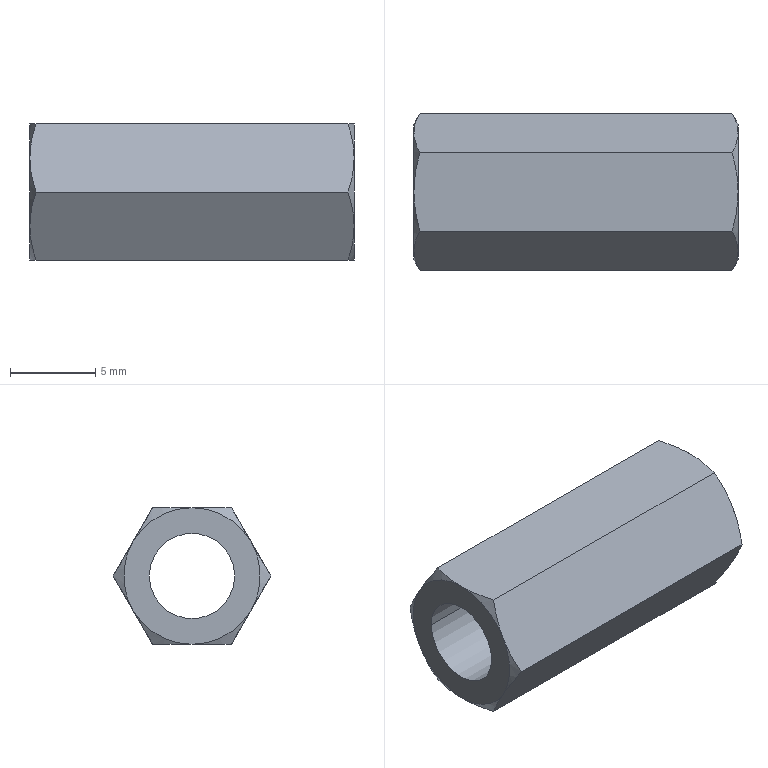Part | STEP file | PLSFB8-19.0-2 | 1 solid | 22 faces | box 19 x 9.238 x 8 mm | volume 678.916 mm3 | cone 12 | plane 8 | cylinder 2 | commonest cylinder face diameters 5 x2
STEP:
#1=CARTESIAN_POINT('',(0.,2.5,0.));
#2=VERTEX_POINT('',#1);
#3=CARTESIAN_POINT('',(0.,-2.5,0.));
#4=VERTEX_POINT('',#3);
#5=CARTESIAN_POINT('',(0.,0.,0.));
#6=DIRECTION('',(1.,0.,0.));
#7=DIRECTION('',(0.,1.,0.));
#8=AXIS2_PLACEMENT_3D('',#5,#6,#7);
#9=CIRCLE('',#8,2.5);
#10=EDGE_CURVE('',#2,#4,#9,.T.);
#11=ORIENTED_EDGE('',*,*,#10,.F.);
#12=CARTESIAN_POINT('',(19.,2.5,0.));
#13=VERTEX_POINT('',#12);
#14=CARTESIAN_POINT('',(19.,2.5,0.));
#15=DIRECTION('',(1.,0.,0.));
#16=VECTOR('',#15,1000.);
#17=LINE('',#14,#16);
#18=EDGE_CURVE('',#2,#13,#17,.T.);
#19=ORIENTED_EDGE('',*,*,#18,.T.);
#20=CARTESIAN_POINT('',(19.,-2.5,0.));
#21=VERTEX_POINT('',#20);
#22=CARTESIAN_POINT('',(19.,0.,0.));
#23=DIRECTION('',(-1.,0.,0.));
#24=DIRECTION('',(0.,-1.,0.));
#25=AXIS2_PLACEMENT_3D('',#22,#23,#24);
#26=CIRCLE('',#25,2.5);
#27=EDGE_CURVE('',#21,#13,#26,.T.);
#28=ORIENTED_EDGE('',*,*,#27,.F.);
#29=CARTESIAN_POINT('',(19.,-2.5,0.));
#30=DIRECTION('',(1.,0.,0.));
#31=VECTOR('',#30,1000.);
#32=LINE('',#29,#31);
#33=EDGE_CURVE('',#4,#21,#32,.T.);
#34=ORIENTED_EDGE('',*,*,#33,.F.);
#35=EDGE_LOOP('',(#11,#19,#28,#34));
#36=FACE_OUTER_BOUND('',#35,.T.);
#37=CARTESIAN_POINT('',(19.,0.,0.));
#38=DIRECTION('',(1.,0.,0.));
#39=DIRECTION('',(0.,-1.,0.));
#40=AXIS2_PLACEMENT_3D('',#37,#38,#39);
#41=CYLINDRICAL_SURFACE('',#40,2.5);
#42=ADVANCED_FACE('',(#36),#41,.F.);
#43=CARTESIAN_POINT('',(18.643,2.309,4.));
#44=VERTEX_POINT('',#43);
#45=CARTESIAN_POINT('',(19.,3.464,2.));
#46=VERTEX_POINT('',#45);
#47=CARTESIAN_POINT('',(18.643,2.309,4.));
#48=CARTESIAN_POINT('',(18.861,2.687,3.346));
#49=CARTESIAN_POINT('',(19.,3.071,2.681));
#50=CARTESIAN_POINT('',(19.,3.464,2.));
#51=B_SPLINE_CURVE_WITH_KNOTS('',3,(#47,#48,#49,#50),.UNSPECIFIED.,.F.,.F.,(4,4),(0.000000238,0.002337),.UNSPECIFIED.);
#52=EDGE_CURVE('',#44,#46,#51,.T.);
#53=ORIENTED_EDGE('',*,*,#52,.T.);
#54=CARTESIAN_POINT('',(18.643,4.619,0.));
#55=VERTEX_POINT('',#54);
#56=CARTESIAN_POINT('',(19.,3.464,2.));
#57=CARTESIAN_POINT('',(19.,3.66,1.661));
#58=CARTESIAN_POINT('',(18.966,3.856,1.322));
#59=CARTESIAN_POINT('',(18.841,4.24,0.6554));
#60=CARTESIAN_POINT('',(18.752,4.43,0.3264));
#61=CARTESIAN_POINT('',(18.643,4.619,0.));
#62=B_SPLINE_CURVE_WITH_KNOTS('',3,(#56,#57,#58,#59,#60,#61),.UNSPECIFIED.,.F.,.F.,(4,2,4),(0.002337,0.003501,0.004665),.UNSPECIFIED.);
#63=EDGE_CURVE('',#46,#55,#62,.T.);
#64=ORIENTED_EDGE('',*,*,#63,.T.);
#65=CARTESIAN_POINT('',(0.3573,4.619,0.));
#66=VERTEX_POINT('',#65);
#67=CARTESIAN_POINT('',(19.,4.619,0.));
#68=DIRECTION('',(-1.,0.,0.));
#69=VECTOR('',#68,1000.);
#70=LINE('',#67,#69);
#71=EDGE_CURVE('',#55,#66,#70,.T.);
#72=ORIENTED_EDGE('',*,*,#71,.T.);
#73=CARTESIAN_POINT('',(0.,3.464,2.));
#74=VERTEX_POINT('',#73);
#75=CARTESIAN_POINT('',(0.3573,4.619,0.));
#76=CARTESIAN_POINT('',(0.1392,4.241,0.6543));
#77=CARTESIAN_POINT('',(0.,3.858,1.319));
#78=CARTESIAN_POINT('',(0.,3.464,2.));
#79=B_SPLINE_CURVE_WITH_KNOTS('',3,(#75,#76,#77,#78),.UNSPECIFIED.,.F.,.F.,(4,4),(0.000000238,0.002337),.UNSPECIFIED.);
#80=EDGE_CURVE('',#66,#74,#79,.T.);
#81=ORIENTED_EDGE('',*,*,#80,.T.);
#82=CARTESIAN_POINT('',(0.3573,2.309,4.));
#83=VERTEX_POINT('',#82);
#84=CARTESIAN_POINT('',(0.,3.464,2.));
#85=CARTESIAN_POINT('',(0.,3.268,2.339));
#86=CARTESIAN_POINT('',(0.03421,3.072,2.678));
#87=CARTESIAN_POINT('',(0.1587,2.688,3.345));
#88=CARTESIAN_POINT('',(0.2485,2.498,3.674));
#89=CARTESIAN_POINT('',(0.3573,2.309,4.));
#90=B_SPLINE_CURVE_WITH_KNOTS('',3,(#84,#85,#86,#87,#88,#89),.UNSPECIFIED.,.F.,.F.,(4,2,4),(0.002337,0.003501,0.004665),.UNSPECIFIED.);
#91=EDGE_CURVE('',#74,#83,#90,.T.);
#92=ORIENTED_EDGE('',*,*,#91,.T.);
#93=CARTESIAN_POINT('',(19.,2.309,4.));
#94=DIRECTION('',(-1.,0.,0.));
#95=VECTOR('',#94,1000.);
#96=LINE('',#93,#95);
#97=EDGE_CURVE('',#44,#83,#96,.T.);
#98=ORIENTED_EDGE('',*,*,#97,.F.);
#99=EDGE_LOOP('',(#53,#64,#72,#81,#92,#98));
#100=FACE_OUTER_BOUND('',#99,.T.);
#101=CARTESIAN_POINT('',(19.,2.309,4.));
#102=DIRECTION('',(0.,-0.866,-0.5));
#103=DIRECTION('',(0.,-0.5,0.866));
#104=AXIS2_PLACEMENT_3D('',#101,#102,#103);
#105=PLANE('',#104);
#106=ADVANCED_FACE('',(#100),#105,.F.);
#107=CARTESIAN_POINT('',(19.,3.464,-2.));
#108=VERTEX_POINT('',#107);
#109=CARTESIAN_POINT('',(18.643,4.619,0.));
#110=CARTESIAN_POINT('',(18.861,4.241,-0.6543));
#111=CARTESIAN_POINT('',(19.,3.858,-1.319));
#112=CARTESIAN_POINT('',(19.,3.464,-2.));
#113=B_SPLINE_CURVE_WITH_KNOTS('',3,(#109,#110,#111,#112),.UNSPECIFIED.,.F.,.F.,(4,4),(0.000000238,0.002337),.UNSPECIFIED.);
#114=EDGE_CURVE('',#55,#108,#113,.T.);
#115=ORIENTED_EDGE('',*,*,#114,.T.);
#116=CARTESIAN_POINT('',(18.643,2.309,-4.));
#117=VERTEX_POINT('',#116);
#118=CARTESIAN_POINT('',(19.,3.464,-2.));
#119=CARTESIAN_POINT('',(19.,3.268,-2.339));
#120=CARTESIAN_POINT('',(18.966,3.072,-2.678));
#121=CARTESIAN_POINT('',(18.841,2.688,-3.345));
#122=CARTESIAN_POINT('',(18.752,2.498,-3.674));
#123=CARTESIAN_POINT('',(18.643,2.309,-4.));
#124=B_SPLINE_CURVE_WITH_KNOTS('',3,(#118,#119,#120,#121,#122,#123),.UNSPECIFIED.,.F.,.F.,(4,2,4),(0.002337,0.003501,0.004665),.UNSPECIFIED.);
#125=EDGE_CURVE('',#108,#117,#124,.T.);
#126=ORIENTED_EDGE('',*,*,#125,.T.);
#127=CARTESIAN_POINT('',(0.3573,2.309,-4.));
#128=VERTEX_POINT('',#127);
#129=CARTESIAN_POINT('',(19.,2.309,-4.));
#130=DIRECTION('',(-1.,0.,0.));
#131=VECTOR('',#130,1000.);
#132=LINE('',#129,#131);
#133=EDGE_CURVE('',#117,#128,#132,.T.);
#134=ORIENTED_EDGE('',*,*,#133,.T.);
#135=CARTESIAN_POINT('',(0.,3.464,-2.));
#136=VERTEX_POINT('',#135);
#137=CARTESIAN_POINT('',(0.3573,2.309,-4.));
#138=CARTESIAN_POINT('',(0.1392,2.687,-3.346));
#139=CARTESIAN_POINT('',(0.,3.071,-2.681));
#140=CARTESIAN_POINT('',(0.,3.464,-2.));
#141=B_SPLINE_CURVE_WITH_KNOTS('',3,(#137,#138,#139,#140),.UNSPECIFIED.,.F.,.F.,(4,4),(0.000000238,0.002337),.UNSPECIFIED.);
#142=EDGE_CURVE('',#128,#136,#141,.T.);
#143=ORIENTED_EDGE('',*,*,#142,.T.);
#144=CARTESIAN_POINT('',(0.,3.464,-2.));
#145=CARTESIAN_POINT('',(0.,3.66,-1.661));
#146=CARTESIAN_POINT('',(0.03421,3.856,-1.322));
#147=CARTESIAN_POINT('',(0.1587,4.24,-0.6554));
#148=CARTESIAN_POINT('',(0.2485,4.43,-0.3264));
#149=CARTESIAN_POINT('',(0.3573,4.619,0.));
#150=B_SPLINE_CURVE_WITH_KNOTS('',3,(#144,#145,#146,#147,#148,#149),.UNSPECIFIED.,.F.,.F.,(4,2,4),(0.002337,0.003501,0.004665),.UNSPECIFIED.);
#151=EDGE_CURVE('',#136,#66,#150,.T.);
#152=ORIENTED_EDGE('',*,*,#151,.T.);
#153=ORIENTED_EDGE('',*,*,#71,.F.);
#154=EDGE_LOOP('',(#115,#126,#134,#143,#152,#153));
#155=FACE_OUTER_BOUND('',#154,.T.);
#156=CARTESIAN_POINT('',(19.,4.619,0.));
#157=DIRECTION('',(0.,-0.866,0.5));
#158=DIRECTION('',(0.,0.5,0.866));
#159=AXIS2_PLACEMENT_3D('',#156,#157,#158);
#160=PLANE('',#159);
#161=ADVANCED_FACE('',(#155),#160,.F.);
#162=CARTESIAN_POINT('',(19.,0.,-4.));
#163=VERTEX_POINT('',#162);
#164=CARTESIAN_POINT('',(18.643,2.309,-4.));
#165=CARTESIAN_POINT('',(18.751,1.934,-4.));
#166=CARTESIAN_POINT('',(18.842,1.549,-4.));
#167=CARTESIAN_POINT('',(18.966,0.778,-4.));
#168=CARTESIAN_POINT('',(19.,0.3903,-4.));
#169=CARTESIAN_POINT('',(19.,0.,-4.));
#170=B_SPLINE_CURVE_WITH_KNOTS('',3,(#164,#165,#166,#167,#168,#169),.UNSPECIFIED.,.F.,.F.,(4,2,4),(0.00412,0.005288,0.006457),.UNSPECIFIED.);
#171=EDGE_CURVE('',#117,#163,#170,.T.);
#172=ORIENTED_EDGE('',*,*,#171,.T.);
#173=CARTESIAN_POINT('',(18.643,-2.309,-4.));
#174=VERTEX_POINT('',#173);
#175=CARTESIAN_POINT('',(19.,0.,-4.));
#176=CARTESIAN_POINT('',(19.,-0.3905,-4.));
#177=CARTESIAN_POINT('',(18.966,-0.7863,-4.));
#178=CARTESIAN_POINT('',(18.84,-1.558,-4.));
#179=CARTESIAN_POINT('',(18.751,-1.936,-4.));
#180=CARTESIAN_POINT('',(18.643,-2.309,-4.));
#181=B_SPLINE_CURVE_WITH_KNOTS('',3,(#175,#176,#177,#178,#179,#180),.UNSPECIFIED.,.F.,.F.,(4,2,4),(0.006457,0.007625,0.008794),.UNSPECIFIED.);
#182=EDGE_CURVE('',#163,#174,#181,.T.);
#183=ORIENTED_EDGE('',*,*,#182,.T.);
#184=CARTESIAN_POINT('',(0.3573,-2.309,-4.));
#185=VERTEX_POINT('',#184);
#186=CARTESIAN_POINT('',(19.,-2.309,-4.));
#187=DIRECTION('',(-1.,0.,0.));
#188=VECTOR('',#187,1000.);
#189=LINE('',#186,#188);
#190=EDGE_CURVE('',#174,#185,#189,.T.);
#191=ORIENTED_EDGE('',*,*,#190,.T.);
#192=CARTESIAN_POINT('',(0.,0.,-4.));
#193=VERTEX_POINT('',#192);
#194=CARTESIAN_POINT('',(0.3573,-2.309,-4.));
#195=CARTESIAN_POINT('',(0.2495,-1.936,-4.));
#196=CARTESIAN_POINT('',(0.1597,-1.558,-4.));
#197=CARTESIAN_POINT('',(0.03447,-0.7863,-4.));
#198=CARTESIAN_POINT('',(0.,-0.3905,-4.));
#199=CARTESIAN_POINT('',(0.,0.,-4.));
#200=B_SPLINE_CURVE_WITH_KNOTS('',3,(#194,#195,#196,#197,#198,#199),.UNSPECIFIED.,.F.,.F.,(4,2,4),(0.001693,0.002859,0.004025),.UNSPECIFIED.);
#201=EDGE_CURVE('',#185,#193,#200,.T.);
#202=ORIENTED_EDGE('',*,*,#201,.T.);
#203=CARTESIAN_POINT('',(0.,0.,-4.));
#204=CARTESIAN_POINT('',(0.,0.3903,-4.));
#205=CARTESIAN_POINT('',(0.03354,0.778,-4.));
#206=CARTESIAN_POINT('',(0.1579,1.549,-4.));
#207=CARTESIAN_POINT('',(0.2488,1.934,-4.));
#208=CARTESIAN_POINT('',(0.3573,2.309,-4.));
#209=B_SPLINE_CURVE_WITH_KNOTS('',3,(#203,#204,#205,#206,#207,#208),.UNSPECIFIED.,.F.,.F.,(4,2,4),(0.004025,0.00519,0.006355),.UNSPECIFIED.);
#210=EDGE_CURVE('',#193,#128,#209,.T.);
#211=ORIENTED_EDGE('',*,*,#210,.T.);
#212=ORIENTED_EDGE('',*,*,#133,.F.);
#213=EDGE_LOOP('',(#172,#183,#191,#202,#211,#212));
#214=FACE_OUTER_BOUND('',#213,.T.);
#215=CARTESIAN_POINT('',(19.,2.309,-4.));
#216=DIRECTION('',(0.,0.,1.));
#217=DIRECTION('',(1.,0.,0.));
#218=AXIS2_PLACEMENT_3D('',#215,#216,#217);
#219=PLANE('',#218);
#220=ADVANCED_FACE('',(#214),#219,.F.);
#221=CARTESIAN_POINT('',(19.,-3.464,-2.));
#222=VERTEX_POINT('',#221);
#223=CARTESIAN_POINT('',(18.643,-2.309,-4.));
#224=CARTESIAN_POINT('',(18.861,-2.687,-3.346));
#225=CARTESIAN_POINT('',(19.,-3.071,-2.681));
#226=CARTESIAN_POINT('',(19.,-3.464,-2.));
#227=B_SPLINE_CURVE_WITH_KNOTS('',3,(#223,#224,#225,#226),.UNSPECIFIED.,.F.,.F.,(4,4),(0.000000238,0.002337),.UNSPECIFIED.);
#228=EDGE_CURVE('',#174,#222,#227,.T.);
#229=ORIENTED_EDGE('',*,*,#228,.T.);
#230=CARTESIAN_POINT('',(18.643,-4.619,0.));
#231=VERTEX_POINT('',#230);
#232=CARTESIAN_POINT('',(19.,-3.464,-2.));
#233=CARTESIAN_POINT('',(19.,-3.66,-1.661));
#234=CARTESIAN_POINT('',(18.966,-3.856,-1.322));
#235=CARTESIAN_POINT('',(18.841,-4.24,-0.6554));
#236=CARTESIAN_POINT('',(18.752,-4.43,-0.3264));
#237=CARTESIAN_POINT('',(18.643,-4.619,0.));
#238=B_SPLINE_CURVE_WITH_KNOTS('',3,(#232,#233,#234,#235,#236,#237),.UNSPECIFIED.,.F.,.F.,(4,2,4),(0.002337,0.003501,0.004665),.UNSPECIFIED.);
#239=EDGE_CURVE('',#222,#231,#238,.T.);
#240=ORIENTED_EDGE('',*,*,#239,.T.);
#241=CARTESIAN_POINT('',(0.3573,-4.619,0.));
#242=VERTEX_POINT('',#241);
#243=CARTESIAN_POINT('',(19.,-4.619,0.));
#244=DIRECTION('',(-1.,0.,0.));
#245=VECTOR('',#244,1000.);
#246=LINE('',#243,#245);
#247=EDGE_CURVE('',#231,#242,#246,.T.);
#248=ORIENTED_EDGE('',*,*,#247,.T.);
#249=CARTESIAN_POINT('',(0.,-3.464,-2.));
#250=VERTEX_POINT('',#249);
#251=CARTESIAN_POINT('',(0.3573,-4.619,0.));
#252=CARTESIAN_POINT('',(0.1392,-4.241,-0.6543));
#253=CARTESIAN_POINT('',(0.,-3.858,-1.319));
#254=CARTESIAN_POINT('',(0.,-3.464,-2.));
#255=B_SPLINE_CURVE_WITH_KNOTS('',3,(#251,#252,#253,#254),.UNSPECIFIED.,.F.,.F.,(4,4),(0.000000238,0.002337),.UNSPECIFIED.);
#256=EDGE_CURVE('',#242,#250,#255,.T.);
#257=ORIENTED_EDGE('',*,*,#256,.T.);
#258=CARTESIAN_POINT('',(0.,-3.464,-2.));
#259=CARTESIAN_POINT('',(0.,-3.268,-2.339));
#260=CARTESIAN_POINT('',(0.03421,-3.072,-2.678));
#261=CARTESIAN_POINT('',(0.1587,-2.688,-3.345));
#262=CARTESIAN_POINT('',(0.2485,-2.498,-3.674));
#263=CARTESIAN_POINT('',(0.3573,-2.309,-4.));
#264=B_SPLINE_CURVE_WITH_KNOTS('',3,(#258,#259,#260,#261,#262,#263),.UNSPECIFIED.,.F.,.F.,(4,2,4),(0.002337,0.003501,0.004665),.UNSPECIFIED.);
#265=EDGE_CURVE('',#250,#185,#264,.T.);
#266=ORIENTED_EDGE('',*,*,#265,.T.);
#267=ORIENTED_EDGE('',*,*,#190,.F.);
#268=EDGE_LOOP('',(#229,#240,#248,#257,#266,#267));
#269=FACE_OUTER_BOUND('',#268,.T.);
#270=CARTESIAN_POINT('',(19.,-2.309,-4.));
#271=DIRECTION('',(0.,0.866,0.5));
#272=DIRECTION('',(0.,0.5,-0.866));
#273=AXIS2_PLACEMENT_3D('',#270,#271,#272);
#274=PLANE('',#273);
#275=ADVANCED_FACE('',(#269),#274,.F.);
#276=CARTESIAN_POINT('',(19.,-3.464,2.));
#277=VERTEX_POINT('',#276);
#278=CARTESIAN_POINT('',(18.643,-4.619,0.));
#279=CARTESIAN_POINT('',(18.861,-4.241,0.6543));
#280=CARTESIAN_POINT('',(19.,-3.858,1.319));
#281=CARTESIAN_POINT('',(19.,-3.464,2.));
#282=B_SPLINE_CURVE_WITH_KNOTS('',3,(#278,#279,#280,#281),.UNSPECIFIED.,.F.,.F.,(4,4),(0.000000238,0.002337),.UNSPECIFIED.);
#283=EDGE_CURVE('',#231,#277,#282,.T.);
#284=ORIENTED_EDGE('',*,*,#283,.T.);
#285=CARTESIAN_POINT('',(18.643,-2.309,4.));
#286=VERTEX_POINT('',#285);
#287=CARTESIAN_POINT('',(19.,-3.464,2.));
#288=CARTESIAN_POINT('',(19.,-3.268,2.339));
#289=CARTESIAN_POINT('',(18.966,-3.072,2.678));
#290=CARTESIAN_POINT('',(18.841,-2.688,3.345));
#291=CARTESIAN_POINT('',(18.752,-2.498,3.674));
#292=CARTESIAN_POINT('',(18.643,-2.309,4.));
#293=B_SPLINE_CURVE_WITH_KNOTS('',3,(#287,#288,#289,#290,#291,#292),.UNSPECIFIED.,.F.,.F.,(4,2,4),(0.002337,0.003501,0.004665),.UNSPECIFIED.);
#294=EDGE_CURVE('',#277,#286,#293,.T.);
#295=ORIENTED_EDGE('',*,*,#294,.T.);
#296=CARTESIAN_POINT('',(0.3573,-2.309,4.));
#297=VERTEX_POINT('',#296);
#298=CARTESIAN_POINT('',(19.,-2.309,4.));
#299=DIRECTION('',(-1.,0.,0.));
#300=VECTOR('',#299,1000.);
#301=LINE('',#298,#300);
#302=EDGE_CURVE('',#286,#297,#301,.T.);
#303=ORIENTED_EDGE('',*,*,#302,.T.);
#304=CARTESIAN_POINT('',(0.,-3.464,2.));
#305=VERTEX_POINT('',#304);
#306=CARTESIAN_POINT('',(0.3573,-2.309,4.));
#307=CARTESIAN_POINT('',(0.1392,-2.687,3.346));
#308=CARTESIAN_POINT('',(0.,-3.071,2.681));
#309=CARTESIAN_POINT('',(0.,-3.464,2.));
#310=B_SPLINE_CURVE_WITH_KNOTS('',3,(#306,#307,#308,#309),.UNSPECIFIED.,.F.,.F.,(4,4),(0.000000238,0.002337),.UNSPECIFIED.);
#311=EDGE_CURVE('',#297,#305,#310,.T.);
#312=ORIENTED_EDGE('',*,*,#311,.T.);
#313=CARTESIAN_POINT('',(0.,-3.464,2.));
#314=CARTESIAN_POINT('',(0.,-3.66,1.661));
#315=CARTESIAN_POINT('',(0.03421,-3.856,1.322));
#316=CARTESIAN_POINT('',(0.1587,-4.24,0.6554));
#317=CARTESIAN_POINT('',(0.2485,-4.43,0.3264));
#318=CARTESIAN_POINT('',(0.3573,-4.619,0.));
#319=B_SPLINE_CURVE_WITH_KNOTS('',3,(#313,#314,#315,#316,#317,#318),.UNSPECIFIED.,.F.,.F.,(4,2,4),(0.002337,0.003501,0.004665),.UNSPECIFIED.);
#320=EDGE_CURVE('',#305,#242,#319,.T.);
#321=ORIENTED_EDGE('',*,*,#320,.T.);
#322=ORIENTED_EDGE('',*,*,#247,.F.);
#323=EDGE_LOOP('',(#284,#295,#303,#312,#321,#322));
#324=FACE_OUTER_BOUND('',#323,.T.);
#325=CARTESIAN_POINT('',(19.,-4.619,0.));
#326=DIRECTION('',(0.,0.866,-0.5));
#327=DIRECTION('',(0.,-0.5,-0.866));
#328=AXIS2_PLACEMENT_3D('',#325,#326,#327);
#329=PLANE('',#328);
#330=ADVANCED_FACE('',(#324),#329,.F.);
#331=CARTESIAN_POINT('',(19.,0.,4.));
#332=VERTEX_POINT('',#331);
#333=CARTESIAN_POINT('',(18.643,-2.309,4.));
#334=CARTESIAN_POINT('',(18.751,-1.936,4.));
#335=CARTESIAN_POINT('',(18.84,-1.558,4.));
#336=CARTESIAN_POINT('',(18.966,-0.7863,4.));
#337=CARTESIAN_POINT('',(19.,-0.3905,4.));
#338=CARTESIAN_POINT('',(19.,0.,4.));
#339=B_SPLINE_CURVE_WITH_KNOTS('',3,(#333,#334,#335,#336,#337,#338),.UNSPECIFIED.,.F.,.F.,(4,2,4),(0.001693,0.002859,0.004025),.UNSPECIFIED.);
#340=EDGE_CURVE('',#286,#332,#339,.T.);
#341=ORIENTED_EDGE('',*,*,#340,.T.);
#342=CARTESIAN_POINT('',(19.,0.,4.));
#343=CARTESIAN_POINT('',(19.,0.3903,4.));
#344=CARTESIAN_POINT('',(18.966,0.778,4.));
#345=CARTESIAN_POINT('',(18.842,1.549,4.));
#346=CARTESIAN_POINT('',(18.751,1.934,4.));
#347=CARTESIAN_POINT('',(18.643,2.309,4.));
#348=B_SPLINE_CURVE_WITH_KNOTS('',3,(#342,#343,#344,#345,#346,#347),.UNSPECIFIED.,.F.,.F.,(4,2,4),(0.004025,0.00519,0.006355),.UNSPECIFIED.);
#349=EDGE_CURVE('',#332,#44,#348,.T.);
#350=ORIENTED_EDGE('',*,*,#349,.T.);
#351=ORIENTED_EDGE('',*,*,#97,.T.);
#352=CARTESIAN_POINT('',(0.,0.,4.));
#353=VERTEX_POINT('',#352);
#354=CARTESIAN_POINT('',(0.3573,2.309,4.));
#355=CARTESIAN_POINT('',(0.2488,1.934,4.));
#356=CARTESIAN_POINT('',(0.1579,1.549,4.));
#357=CARTESIAN_POINT('',(0.03354,0.778,4.));
#358=CARTESIAN_POINT('',(0.,0.3903,4.));
#359=CARTESIAN_POINT('',(0.,0.,4.));
#360=B_SPLINE_CURVE_WITH_KNOTS('',3,(#354,#355,#356,#357,#358,#359),.UNSPECIFIED.,.F.,.F.,(4,2,4),(0.00412,0.005288,0.006457),.UNSPECIFIED.);
#361=EDGE_CURVE('',#83,#353,#360,.T.);
#362=ORIENTED_EDGE('',*,*,#361,.T.);
#363=CARTESIAN_POINT('',(0.,0.,4.));
#364=CARTESIAN_POINT('',(0.,-0.3905,4.));
#365=CARTESIAN_POINT('',(0.03447,-0.7863,4.));
#366=CARTESIAN_POINT('',(0.1597,-1.558,4.));
#367=CARTESIAN_POINT('',(0.2495,-1.936,4.));
#368=CARTESIAN_POINT('',(0.3573,-2.309,4.));
#369=B_SPLINE_CURVE_WITH_KNOTS('',3,(#363,#364,#365,#366,#367,#368),.UNSPECIFIED.,.F.,.F.,(4,2,4),(0.006457,0.007625,0.008794),.UNSPECIFIED.);
#370=EDGE_CURVE('',#353,#297,#369,.T.);
#371=ORIENTED_EDGE('',*,*,#370,.T.);
#372=ORIENTED_EDGE('',*,*,#302,.F.);
#373=EDGE_LOOP('',(#341,#350,#351,#362,#371,#372));
#374=FACE_OUTER_BOUND('',#373,.T.);
#375=CARTESIAN_POINT('',(19.,-2.309,4.));
#376=DIRECTION('',(0.,0.,-1.));
#377=DIRECTION('',(-1.,0.,0.));
#378=AXIS2_PLACEMENT_3D('',#375,#376,#377);
#379=PLANE('',#378);
#380=ADVANCED_FACE('',(#374),#379,.F.);
#381=ORIENTED_EDGE('',*,*,#210,.F.);
#382=CARTESIAN_POINT('',(0.,0.,0.));
#383=DIRECTION('',(-1.,0.,0.));
#384=DIRECTION('',(0.,0.,-1.));
#385=AXIS2_PLACEMENT_3D('',#382,#383,#384);
#386=CIRCLE('',#385,4.);
#387=EDGE_CURVE('',#136,#193,#386,.T.);
#388=ORIENTED_EDGE('',*,*,#387,.F.);
#389=ORIENTED_EDGE('',*,*,#142,.F.);
#390=EDGE_LOOP('',(#381,#388,#389));
#391=FACE_OUTER_BOUND('',#390,.T.);
#392=CARTESIAN_POINT('',(0.,0.,0.));
#393=DIRECTION('',(1.,0.,0.));
#394=DIRECTION('',(0.,0.,-1.));
#395=AXIS2_PLACEMENT_3D('',#392,#393,#394);
#396=CONICAL_SURFACE('',#395,4.,1.047);
#397=ADVANCED_FACE('',(#391),#396,.T.);
#398=ORIENTED_EDGE('',*,*,#151,.F.);
#399=CARTESIAN_POINT('',(0.,0.,0.));
#400=DIRECTION('',(-1.,0.,0.));
#401=DIRECTION('',(0.,0.,-1.));
#402=AXIS2_PLACEMENT_3D('',#399,#400,#401);
#403=CIRCLE('',#402,4.);
#404=EDGE_CURVE('',#74,#136,#403,.T.);
#405=ORIENTED_EDGE('',*,*,#404,.F.);
#406=ORIENTED_EDGE('',*,*,#80,.F.);
#407=EDGE_LOOP('',(#398,#405,#406));
#408=FACE_OUTER_BOUND('',#407,.T.);
#409=CARTESIAN_POINT('',(0.,0.,0.));
#410=DIRECTION('',(1.,0.,0.));
#411=DIRECTION('',(0.,0.,-1.));
#412=AXIS2_PLACEMENT_3D('',#409,#410,#411);
#413=CONICAL_SURFACE('',#412,4.,1.047);
#414=ADVANCED_FACE('',(#408),#413,.T.);
#415=ORIENTED_EDGE('',*,*,#91,.F.);
#416=CARTESIAN_POINT('',(0.,0.,0.));
#417=DIRECTION('',(-1.,0.,0.));
#418=DIRECTION('',(0.,0.,-1.));
#419=AXIS2_PLACEMENT_3D('',#416,#417,#418);
#420=CIRCLE('',#419,4.);
#421=EDGE_CURVE('',#353,#74,#420,.T.);
#422=ORIENTED_EDGE('',*,*,#421,.F.);
#423=ORIENTED_EDGE('',*,*,#361,.F.);
#424=EDGE_LOOP('',(#415,#422,#423));
#425=FACE_OUTER_BOUND('',#424,.T.);
#426=CARTESIAN_POINT('',(0.,0.,0.));
#427=DIRECTION('',(1.,0.,0.));
#428=DIRECTION('',(0.,0.,-1.));
#429=AXIS2_PLACEMENT_3D('',#426,#427,#428);
#430=CONICAL_SURFACE('',#429,4.,1.047);
#431=ADVANCED_FACE('',(#425),#430,.T.);
#432=ORIENTED_EDGE('',*,*,#311,.F.);
#433=ORIENTED_EDGE('',*,*,#370,.F.);
#434=CARTESIAN_POINT('',(0.,0.,0.));
#435=DIRECTION('',(1.,0.,0.));
#436=DIRECTION('',(0.,0.,1.));
#437=AXIS2_PLACEMENT_3D('',#434,#435,#436);
#438=CIRCLE('',#437,4.);
#439=EDGE_CURVE('',#353,#305,#438,.T.);
#440=ORIENTED_EDGE('',*,*,#439,.T.);
#441=EDGE_LOOP('',(#432,#433,#440));
#442=FACE_OUTER_BOUND('',#441,.T.);
#443=CARTESIAN_POINT('',(0.,0.,0.));
#444=DIRECTION('',(1.,0.,0.));
#445=DIRECTION('',(0.,0.,-1.));
#446=AXIS2_PLACEMENT_3D('',#443,#444,#445);
#447=CONICAL_SURFACE('',#446,4.,1.047);
#448=ADVANCED_FACE('',(#442),#447,.T.);
#449=ORIENTED_EDGE('',*,*,#256,.F.);
#450=ORIENTED_EDGE('',*,*,#320,.F.);
#451=CARTESIAN_POINT('',(0.,0.,0.));
#452=DIRECTION('',(-1.,0.,0.));
#453=DIRECTION('',(0.,0.,-1.));
#454=AXIS2_PLACEMENT_3D('',#451,#452,#453);
#455=CIRCLE('',#454,4.);
#456=EDGE_CURVE('',#250,#305,#455,.T.);
#457=ORIENTED_EDGE('',*,*,#456,.F.);
#458=EDGE_LOOP('',(#449,#450,#457));
#459=FACE_OUTER_BOUND('',#458,.T.);
#460=CARTESIAN_POINT('',(0.,0.,0.));
#461=DIRECTION('',(1.,0.,0.));
#462=DIRECTION('',(0.,0.,-1.));
#463=AXIS2_PLACEMENT_3D('',#460,#461,#462);
#464=CONICAL_SURFACE('',#463,4.,1.047);
#465=ADVANCED_FACE('',(#459),#464,.T.);
#466=ORIENTED_EDGE('',*,*,#201,.F.);
#467=ORIENTED_EDGE('',*,*,#265,.F.);
#468=CARTESIAN_POINT('',(0.,0.,0.));
#469=DIRECTION('',(-1.,0.,0.));
#470=DIRECTION('',(0.,0.,-1.));
#471=AXIS2_PLACEMENT_3D('',#468,#469,#470);
#472=CIRCLE('',#471,4.);
#473=EDGE_CURVE('',#193,#250,#472,.T.);
#474=ORIENTED_EDGE('',*,*,#473,.F.);
#475=EDGE_LOOP('',(#466,#467,#474));
#476=FACE_OUTER_BOUND('',#475,.T.);
#477=CARTESIAN_POINT('',(0.,0.,0.));
#478=DIRECTION('',(1.,0.,0.));
#479=DIRECTION('',(0.,0.,-1.));
#480=AXIS2_PLACEMENT_3D('',#477,#478,#479);
#481=CONICAL_SURFACE('',#480,4.,1.047);
#482=ADVANCED_FACE('',(#476),#481,.T.);
#483=CARTESIAN_POINT('',(0.,0.,0.));
#484=DIRECTION('',(1.,0.,0.));
#485=DIRECTION('',(0.,1.,0.));
#486=AXIS2_PLACEMENT_3D('',#483,#484,#485);
#487=CIRCLE('',#486,2.5);
#488=EDGE_CURVE('',#4,#2,#487,.T.);
#489=ORIENTED_EDGE('',*,*,#488,.T.);
#490=ORIENTED_EDGE('',*,*,#10,.T.);
#491=EDGE_LOOP('',(#489,#490));
#492=FACE_BOUND('',#491,.T.);
#493=ORIENTED_EDGE('',*,*,#473,.T.);
#494=ORIENTED_EDGE('',*,*,#456,.T.);
#495=ORIENTED_EDGE('',*,*,#439,.F.);
#496=ORIENTED_EDGE('',*,*,#421,.T.);
#497=ORIENTED_EDGE('',*,*,#404,.T.);
#498=ORIENTED_EDGE('',*,*,#387,.T.);
#499=EDGE_LOOP('',(#493,#494,#495,#496,#497,#498));
#500=FACE_OUTER_BOUND('',#499,.T.);
#501=CARTESIAN_POINT('',(0.,0.,0.));
#502=DIRECTION('',(1.,0.,0.));
#503=DIRECTION('',(0.,0.,-1.));
#504=AXIS2_PLACEMENT_3D('',#501,#502,#503);
#505=PLANE('',#504);
#506=ADVANCED_FACE('',(#492,#500),#505,.F.);
#507=ORIENTED_EDGE('',*,*,#125,.F.);
#508=CARTESIAN_POINT('',(19.,0.,0.));
#509=DIRECTION('',(-1.,0.,0.));
#510=DIRECTION('',(0.,0.,-1.));
#511=AXIS2_PLACEMENT_3D('',#508,#509,#510);
#512=CIRCLE('',#511,4.);
#513=EDGE_CURVE('',#108,#163,#512,.T.);
#514=ORIENTED_EDGE('',*,*,#513,.T.);
#515=ORIENTED_EDGE('',*,*,#171,.F.);
#516=EDGE_LOOP('',(#507,#514,#515));
#517=FACE_OUTER_BOUND('',#516,.T.);
#518=CARTESIAN_POINT('',(18.643,0.,0.));
#519=DIRECTION('',(-1.,0.,0.));
#520=DIRECTION('',(0.,0.,1.));
#521=AXIS2_PLACEMENT_3D('',#518,#519,#520);
#522=CONICAL_SURFACE('',#521,4.619,1.047);
#523=ADVANCED_FACE('',(#517),#522,.T.);
#524=ORIENTED_EDGE('',*,*,#63,.F.);
#525=CARTESIAN_POINT('',(19.,0.,0.));
#526=DIRECTION('',(-1.,0.,0.));
#527=DIRECTION('',(0.,0.,-1.));
#528=AXIS2_PLACEMENT_3D('',#525,#526,#527);
#529=CIRCLE('',#528,4.);
#530=EDGE_CURVE('',#46,#108,#529,.T.);
#531=ORIENTED_EDGE('',*,*,#530,.T.);
#532=ORIENTED_EDGE('',*,*,#114,.F.);
#533=EDGE_LOOP('',(#524,#531,#532));
#534=FACE_OUTER_BOUND('',#533,.T.);
#535=CARTESIAN_POINT('',(18.643,0.,0.));
#536=DIRECTION('',(-1.,0.,0.));
#537=DIRECTION('',(0.,0.,1.));
#538=AXIS2_PLACEMENT_3D('',#535,#536,#537);
#539=CONICAL_SURFACE('',#538,4.619,1.047);
#540=ADVANCED_FACE('',(#534),#539,.T.);
#541=ORIENTED_EDGE('',*,*,#52,.F.);
#542=ORIENTED_EDGE('',*,*,#349,.F.);
#543=CARTESIAN_POINT('',(19.,0.,0.));
#544=DIRECTION('',(-1.,0.,0.));
#545=DIRECTION('',(0.,0.,-1.));
#546=AXIS2_PLACEMENT_3D('',#543,#544,#545);
#547=CIRCLE('',#546,4.);
#548=EDGE_CURVE('',#332,#46,#547,.T.);
#549=ORIENTED_EDGE('',*,*,#548,.T.);
#550=EDGE_LOOP('',(#541,#542,#549));
#551=FACE_OUTER_BOUND('',#550,.T.);
#552=CARTESIAN_POINT('',(18.643,0.,0.));
#553=DIRECTION('',(-1.,0.,0.));
#554=DIRECTION('',(0.,0.,1.));
#555=AXIS2_PLACEMENT_3D('',#552,#553,#554);
#556=CONICAL_SURFACE('',#555,4.619,1.047);
#557=ADVANCED_FACE('',(#551),#556,.T.);
#558=ORIENTED_EDGE('',*,*,#294,.F.);
#559=CARTESIAN_POINT('',(19.,0.,0.));
#560=DIRECTION('',(1.,0.,0.));
#561=DIRECTION('',(0.,0.,1.));
#562=AXIS2_PLACEMENT_3D('',#559,#560,#561);
#563=CIRCLE('',#562,4.);
#564=EDGE_CURVE('',#332,#277,#563,.T.);
#565=ORIENTED_EDGE('',*,*,#564,.F.);
#566=ORIENTED_EDGE('',*,*,#340,.F.);
#567=EDGE_LOOP('',(#558,#565,#566));
#568=FACE_OUTER_BOUND('',#567,.T.);
#569=CARTESIAN_POINT('',(18.643,0.,0.));
#570=DIRECTION('',(-1.,0.,0.));
#571=DIRECTION('',(0.,0.,1.));
#572=AXIS2_PLACEMENT_3D('',#569,#570,#571);
#573=CONICAL_SURFACE('',#572,4.619,1.047);
#574=ADVANCED_FACE('',(#568),#573,.T.);
#575=ORIENTED_EDGE('',*,*,#239,.F.);
#576=CARTESIAN_POINT('',(19.,0.,0.));
#577=DIRECTION('',(-1.,0.,0.));
#578=DIRECTION('',(0.,0.,-1.));
#579=AXIS2_PLACEMENT_3D('',#576,#577,#578);
#580=CIRCLE('',#579,4.);
#581=EDGE_CURVE('',#222,#277,#580,.T.);
#582=ORIENTED_EDGE('',*,*,#581,.T.);
#583=ORIENTED_EDGE('',*,*,#283,.F.);
#584=EDGE_LOOP('',(#575,#582,#583));
#585=FACE_OUTER_BOUND('',#584,.T.);
#586=CARTESIAN_POINT('',(18.643,0.,0.));
#587=DIRECTION('',(-1.,0.,0.));
#588=DIRECTION('',(0.,0.,1.));
#589=AXIS2_PLACEMENT_3D('',#586,#587,#588);
#590=CONICAL_SURFACE('',#589,4.619,1.047);
#591=ADVANCED_FACE('',(#585),#590,.T.);
#592=ORIENTED_EDGE('',*,*,#182,.F.);
#593=CARTESIAN_POINT('',(19.,0.,0.));
#594=DIRECTION('',(-1.,0.,0.));
#595=DIRECTION('',(0.,0.,-1.));
#596=AXIS2_PLACEMENT_3D('',#593,#594,#595);
#597=CIRCLE('',#596,4.);
#598=EDGE_CURVE('',#163,#222,#597,.T.);
#599=ORIENTED_EDGE('',*,*,#598,.T.);
#600=ORIENTED_EDGE('',*,*,#228,.F.);
#601=EDGE_LOOP('',(#592,#599,#600));
#602=FACE_OUTER_BOUND('',#601,.T.);
#603=CARTESIAN_POINT('',(18.643,0.,0.));
#604=DIRECTION('',(-1.,0.,0.));
#605=DIRECTION('',(0.,0.,1.));
#606=AXIS2_PLACEMENT_3D('',#603,#604,#605);
#607=CONICAL_SURFACE('',#606,4.619,1.047);
#608=ADVANCED_FACE('',(#602),#607,.T.);
#609=ORIENTED_EDGE('',*,*,#27,.T.);
#610=CARTESIAN_POINT('',(19.,0.,0.));
#611=DIRECTION('',(-1.,0.,0.));
#612=DIRECTION('',(0.,-1.,0.));
#613=AXIS2_PLACEMENT_3D('',#610,#611,#612);
#614=CIRCLE('',#613,2.5);
#615=EDGE_CURVE('',#13,#21,#614,.T.);
#616=ORIENTED_EDGE('',*,*,#615,.T.);
#617=EDGE_LOOP('',(#609,#616));
#618=FACE_BOUND('',#617,.T.);
#619=ORIENTED_EDGE('',*,*,#513,.F.);
#620=ORIENTED_EDGE('',*,*,#530,.F.);
#621=ORIENTED_EDGE('',*,*,#548,.F.);
#622=ORIENTED_EDGE('',*,*,#564,.T.);
#623=ORIENTED_EDGE('',*,*,#581,.F.);
#624=ORIENTED_EDGE('',*,*,#598,.F.);
#625=EDGE_LOOP('',(#619,#620,#621,#622,#623,#624));
#626=FACE_OUTER_BOUND('',#625,.T.);
#627=CARTESIAN_POINT('',(19.,0.,0.));
#628=DIRECTION('',(1.,0.,0.));
#629=DIRECTION('',(0.,0.,-1.));
#630=AXIS2_PLACEMENT_3D('',#627,#628,#629);
#631=PLANE('',#630);
#632=ADVANCED_FACE('',(#618,#626),#631,.T.);
#633=ORIENTED_EDGE('',*,*,#18,.F.);
#634=ORIENTED_EDGE('',*,*,#488,.F.);
#635=ORIENTED_EDGE('',*,*,#33,.T.);
#636=ORIENTED_EDGE('',*,*,#615,.F.);
#637=EDGE_LOOP('',(#633,#634,#635,#636));
#638=FACE_OUTER_BOUND('',#637,.T.);
#639=CARTESIAN_POINT('',(19.,0.,0.));
#640=DIRECTION('',(1.,0.,0.));
#641=DIRECTION('',(0.,-1.,0.));
#642=AXIS2_PLACEMENT_3D('',#639,#640,#641);
#643=CYLINDRICAL_SURFACE('',#642,2.5);
#644=ADVANCED_FACE('',(#638),#643,.F.);
#645=CLOSED_SHELL('',(#42,#106,#161,#220,#275,#330,#380,#397,#414,#431,#448,#465,#482,#506,#523,#540,#557,#574,#591,#608,#632,#644));
#646=MANIFOLD_SOLID_BREP('',#645);
#647=CARTESIAN_POINT('',(0.,0.,0.));
#648=DIRECTION('',(0.,0.,1.));
#649=DIRECTION('',(1.,0.,0.));
#650=AXIS2_PLACEMENT_3D('',#647,#648,#649);
#651=(LENGTH_UNIT()NAMED_UNIT(*)SI_UNIT(.MILLI.,.METRE.));
#652=UNCERTAINTY_MEASURE_WITH_UNIT(LENGTH_MEASURE(0.00001),#651,'','');
#653=(NAMED_UNIT(*)PLANE_ANGLE_UNIT()SI_UNIT($,.RADIAN.));
#654=(NAMED_UNIT(*)SI_UNIT($,.STERADIAN.)SOLID_ANGLE_UNIT());
#655=(GEOMETRIC_REPRESENTATION_CONTEXT(3)GLOBAL_UNCERTAINTY_ASSIGNED_CONTEXT((#652))GLOBAL_UNIT_ASSIGNED_CONTEXT((#651,#653,#654))REPRESENTATION_CONTEXT('',''));
#656=ADVANCED_BREP_SHAPE_REPRESENTATION('',(#646,#650),#655);